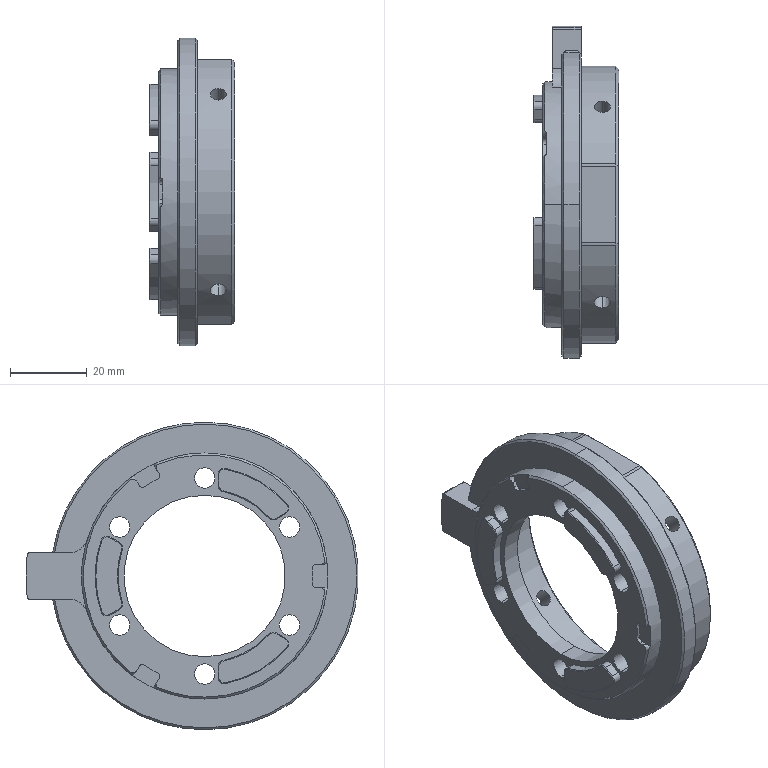NC program | NX | posted with a generic post | part box 22.3 x 86.5 x 80 mm
Lines 2663 to 3025 of 3025:
(PLANAR_MILL_COPY_COPY_COPY_COPY_COPY_COPY_1_COPY_1 , TOOL : D6A45)
N5282 T01 M6
N5284 G54
N5286 G17 G0 G90 X-1.7 Y25.849 S9500 M3
N5288 G43 Z30. H1
N5290 Z0.
N5292 G94 G1 Z-1.5 F1250.
N5294 G3 X-2.2 Y24.983 R1.
N5296 G1 Y23.554
N5298 G2 X-4.486 Y20.72 R2.9
N5300 G3 X-15.701 Y14.245 R21.2
N5302 G2 X-19.299 Y13.682 R2.9
N5304 G1 X-21.774 Y15.111
N5306 G2 X-22.515 Y19.523 R2.9
N5308 X-5.65 Y29.26 R29.8
N5310 X-2.2 Y26.412 R2.9
N5312 G1 Y24.983
N5314 G3 X-1.7 Y24.117 R1.
N5316 G1 Z0.
N5318 G0 Z30.
N5320 X-21.536 Y-14.397
N5322 Z0.
N5324 G1 Z-1.5
N5326 G3 X-20.536 Y-14.397 R1.
N5328 G1 X-19.299 Y-13.682
N5330 G2 X-15.701 Y-14.245 R2.9
N5332 G3 X-4.486 Y-20.72 R21.2
N5334 G2 X-2.2 Y-23.554 R2.9
N5336 G1 Y-26.412
N5338 G2 X-5.65 Y-29.26 R2.9
N5340 X-22.515 Y-19.523 R29.8
N5342 X-21.774 Y-15.111 R2.9
N5344 G1 X-20.536 Y-14.397
N5346 G3 X-20.036 Y-13.531 R1.
N5348 G1 Z0.
N5350 G0 Z30.
N5352 X23.236 Y-11.452
N5354 Z0.
N5356 G1 Z-1.5
N5358 G3 X22.736 Y-10.586 R1.
N5360 G1 X21.499 Y-9.872
N5362 G2 X20.187 Y-6.475 R2.9
N5364 G3 X20.187 Y6.475 R21.2
N5366 G2 X21.499 Y9.872 R2.9
N5368 G1 X23.974 Y11.301
N5370 G2 X28.164 Y9.737 R2.9
N5372 X28.164 Y-9.737 R29.8
N5374 X23.974 Y-11.301 R2.9
N5376 G1 X22.736 Y-10.586
N5378 G3 X21.736 Y-10.586 R1.
N5380 G1 Z0.
N5382 G0 Z30.
(PLANAR_MILL_COPY_COPY_COPY_COPY_COPY_COPY_1_COPY_1_COPY , TOOL : D6A45)
N5384 X13.9 Y25.808
N5386 Z-1.8
N5388 G1 Z-3.3
N5390 G3 X14.4 Y24.942 R1.
N5392 G2 X16.086 Y23.889 R28.8
N5394 G3 X16.371 Y23.955 R0.2
N5396 G1 X16.815 Y24.724
N5398 G2 X17.223 Y25.267 R2.834
N5400 X17.805 Y25.712 R2.371
N5402 X18.641 Y25.948 R1.983
N5404 X19.647 Y25.638 R1.517
N5406 X19.647 Y-25.638 R32.3
N5408 X18.64 Y-25.948 R1.517
N5410 X17.805 Y-25.712 R1.984
N5412 X17.222 Y-25.267 R2.37
N5414 X16.815 Y-24.724 R2.835
N5416 G1 X16.371 Y-23.955
N5418 G3 X16.086 Y-23.889 R0.2
N5420 G2 X12.646 Y-25.875 R28.8
N5422 G3 X12.56 Y-26.155 R0.2
N5424 G1 X13.004 Y-26.924
N5426 G2 X13.271 Y-27.549 R2.834
N5428 X13.365 Y-28.276 R2.371
N5430 X13.152 Y-29.117 R1.983
N5432 X12.38 Y-29.833 R1.517
N5434 X-32.026 Y-4.196 R32.3
N5436 X-31.792 Y-3.169 R1.517
N5438 X-31.17 Y-2.564 R1.984
N5440 X-30.493 Y-2.281 R2.37
N5442 X-29.819 Y-2.2 R2.835
N5444 G1 X-28.931
N5446 G3 X-28.731 Y-1.986 R0.2
N5448 G2 X-28.731 Y1.986 R28.8
N5450 G3 X-28.931 Y2.2 R0.2
N5452 G1 X-29.819
N5454 G2 X-30.494 Y2.282 R2.834
N5456 X-31.17 Y2.564 R2.371
N5458 X-31.792 Y3.169 R1.983
N5460 X-32.026 Y4.196 R1.517
N5462 X12.38 Y29.833 R32.3
N5464 X13.152 Y29.117 R1.517
N5466 X13.365 Y28.275 R1.984
N5468 X13.271 Y27.549 R2.37
N5470 X13.004 Y26.924 R2.835
N5472 G1 X12.56 Y26.155
N5474 G3 X12.646 Y25.875 R0.2
N5476 G2 X14.4 Y24.942 R28.8
N5478 G3 X15.4 Y24.942 R1.
N5480 G1 Z-1.8
N5482 G0 Z30.
(PLANAR_MILL_COPY_COPY_COPY_COPY_COPY_COPY_1_COPY_1_COPY_1 , TOOL : D6A45)
N5484 X1.198 Y25.871
N5486 Z-2.5
N5488 G1 X0.905 Y26.405 Z-2.663
N5490 X0.276 Y26.75 Z-2.855
N5492 X-0.006 Z-2.934
N5494 X0.276 Z-3.009
N5496 X0.905 Y26.405 Z-3.201
N5498 X1.25 Y25.776 Z-3.394
N5500 Y25.225 Z-3.541
N5502 X0.905 Y24.595 Z-3.734
N5504 X0.276 Y24.25 Z-3.926
N5506 X0. Z-4.
N5508 G3 X1.25 Y25.5 R1.25
N5510 X-0.011 Y26.75 R1.25
N5512 X0.545 Y25.919 R1.
N5514 G1 Z-2.5
N5516 G0 Z30.
N5518 X21.151 Y13.604
N5520 Z-2.5
N5522 G1 X20.834 Y13.026 Z-2.677
N5524 X20.863 Y12.364 Z-2.855
N5526 X21.001 Y12.125 Z-2.929
N5528 X20.863 Y12.364 Z-3.003
N5530 X20.834 Y12.475 Z-3.034
N5532 Y12.75 Z-3.107
N5534 Y13.026 Z-3.181
N5536 X21.179 Y13.655 Z-3.374
N5538 X21.808 Y14. Z-3.566
N5540 X22.359 Z-3.714
N5542 X22.729 Y13.856 Z-3.82
N5544 X23.036 Y13.605 Z-3.926
N5546 X23.172 Y13.365 Z-4.
N5548 G3 X21.468 Y13.838 R1.25
N5550 X21.001 Y12.125 R1.25
N5552 X21.501 Y12.991 R1.
N5554 G1 Z-2.5
N5556 G0 Z30.
N5558 X16.662 Y6.951
N5560 Z-2.5
N5562 G1 Z-4.
N5564 X17.284 Y7.212
N5566 G3 X17.89 Y8.007 R1.
N5568 X-2.01 Y19.497 R19.6
N5570 X-2.396 Y18.574 R1.
N5572 G1 X-2.311 Y17.905
N5574 Z-2.5
N5576 G0 Z30.
N5578 X-14.351 Y10.954
N5580 Z-2.5
N5582 G1 Z-4.
N5584 X-14.888 Y11.362
N5586 G3 X-15.879 Y11.489 R1.
N5588 X-15.879 Y-11.489 R19.6
N5590 X-14.888 Y-11.362 R1.
N5592 G1 X-14.351 Y-10.954
N5594 Z-2.5
N5596 G0 Z30.
N5598 X-2.311 Y-17.905
N5600 Z-2.5
N5602 G1 Z-4.
N5604 X-2.396 Y-18.574
N5606 G3 X-2.01 Y-19.497 R1.
N5608 X17.89 Y-8.007 R19.6
N5610 X17.284 Y-7.212 R1.
N5612 G1 X16.662 Y-6.951
N5614 Z-2.5
N5616 G0 Z30.
N5618 X21.827 Y-14.
N5620 Z-2.5
N5622 G1 X22.359 Z-2.643
N5624 X22.729 Y-13.856 Z-2.749
N5626 X23.036 Y-13.605 Z-2.855
N5628 X23.172 Y-13.365 Z-2.929
N5630 X23.036 Y-13.605 Z-3.003
N5632 X22.729 Y-13.856 Z-3.109
N5634 X22.359 Y-14. Z-3.215
N5636 X21.808 Z-3.363
N5638 X21.179 Y-13.655 Z-3.555
N5640 X20.834 Y-13.026 Z-3.748
N5642 X20.863 Y-12.364 Z-3.926
N5644 X21.001 Y-12.125 Z-4.
N5646 G3 X21.459 Y-13.833 R1.25
N5648 X23.172 Y-13.365 R1.25
N5650 X22.174 Y-13.432 R1.
N5652 G1 Z-2.5
N5654 G0 Z30.
N5656 X1.203 Y-25.139
N5658 Z-2.5
N5660 G1 X0.905 Y-24.595 Z-2.666
N5662 X0.276 Y-24.25 Z-2.858
N5664 X0. Z-2.932
N5666 X0.276 Z-3.006
N5668 X0.905 Y-24.595 Z-3.198
N5670 X1.25 Y-25.225 Z-3.391
N5672 Y-25.776 Z-3.538
N5674 X0.905 Y-26.405 Z-3.731
N5676 X0.276 Y-26.75 Z-3.923
N5678 X-0.011 Z-4.
N5680 G3 X1.25 Y-25.511 R1.25
N5682 X0. Y-24.25 R1.25
N5684 X0.5 Y-25.116 R1.
N5686 G1 Z-2.5
N5688 G0 Z30.
N5690 X-23.018 Y-11.898
N5692 Z-2.5
N5694 G1 X-23.334 Y-12.475 Z-2.676
N5696 X-23.3 Y-13.147 Z-2.858
N5698 X-23.161 Y-13.385 Z-2.931
N5700 X-23.3 Y-13.147 Z-3.005
N5702 X-23.334 Y-13.026 Z-3.039
N5704 Y-12.475 Z-3.187
N5706 X-22.989 Y-11.845 Z-3.379
N5708 X-22.359 Y-11.5 Z-3.571
N5710 X-21.808 Z-3.719
N5712 X-21.139 Y-11.886 Z-3.926
N5714 X-21.001 Y-12.125 Z-4.
N5716 G3 X-22.709 Y-11.667 R1.25
N5718 X-23.161 Y-13.385 R1.25
N5720 X-22.719 Y-12.487 R1.
N5722 G1 Z-2.5
N5724 G0 Z30.
N5726 X-22.369 Y11.505
N5728 Z-2.5
N5730 G1 X-21.808 Y11.5 Z-2.651
N5732 X-21.139 Y11.886 Z-2.858
N5734 X-21.001 Y12.125 Z-2.931
N5736 X-21.139 Y11.886 Z-3.005
N5738 X-21.808 Y11.5 Z-3.212
N5740 X-22.359 Z-3.36
N5742 X-22.989 Y11.845 Z-3.552
N5744 X-23.334 Y12.475 Z-3.745
N5746 X-23.3 Y13.147 Z-3.926
N5748 X-23.161 Y13.385 Z-4.
N5750 G3 X-22.718 Y11.673 R1.25
N5752 X-21.001 Y12.125 R1.25
N5754 X-22.001 Y12.125 R1.
N5756 G1 Z-2.5
N5758 G0 Z30.
(DRILLING_COPY_1 , TOOL : D6A45)
N5760 X-22.084 Y12.75 S5000
N5762 G81 G98 Z-5.25 F350. R0.5
N5764 Y-12.75
N5766 X0. Y-25.5
N5768 X22.084 Y-12.75
N5770 Y12.75
N5772 X0. Y25.5
N5774 G80
N5776 G0 X0. Y25.5 Z30.
(PLANAR_MILL_COPY_COPY_COPY_COPY_COPY_COPY_1_COPY_1_COPY_2 , TOOL : D6A45)
N5778 X40.64 Y-10.7 S9500
N5780 Z-7.
N5782 G1 Z-8.5 F1250.
N5784 X40.236 Y-10.
N5786 G3 X39.37 Y-9.5 R1.
N5788 G2 X39.37 Y9.5 R-40.5
N5790 G3 X40.236 Y10. R1.
N5792 G1 X40.64 Y10.7
N5794 Z-7.
N5796 G0 Z30.
(PLANAR_MILL_COPY_COPY_COPY_COPY_COPY_COPY_1_COPY_1_COPY_1_COPY , TOOL : D6A45)
N5798 X35.597 Y8.931
N5800 Z-5.
N5802 G1 Z-6.5
N5804 X35.016 Y8.405
N5806 G3 X34.709 Y7.453 R1.
N5808 X35.327 Y7.4 R3.6
N5810 G1 X45.659
N5812 G2 X47.544 Y5.735 R1.9
N5814 X47.544 Y-5.735 R46.4
N5816 X45.659 Y-7.4 R1.9
N5818 G1 X35.327
N5820 G3 X34.709 Y-7.453 R3.6
N5822 X35.016 Y-8.405 R1.
N5824 G1 X35.597 Y-8.931
N5826 Z-5.
N5828 G0 Z30.
N5830 M5
(TOOLCOMP14_COPY , TOOL : D10JING)
N5832 T14 M6
N5834 G54
N5836 G17 G0 G90 X-7.721 Y33.774 S9500 M3
N5838 G43 Z30. H14
N5840 Z-1.5
N5842 G94 G1 Z-2.5 F1250.
N5844 G41 X-7.67 Y33.688 D14
N5846 X-7.306 Y33.268
N5848 G3 X-6.361 Y32.942 R1.
N5850 G2 X1.55 Y26.412 R6.65
N5852 G1 Y23.554
N5854 G2 X-3.693 Y17.055 R6.65
N5856 G3 X-12.924 Y11.725 R17.45
N5858 G2 X-21.174 Y10.435 R6.65
N5860 G1 X-23.649 Y11.864
N5862 G2 X-25.348 Y21.979 R6.65
N5864 X-6.361 Y32.942 R33.55
N5866 G3 X-5.605 Y33.597 R1.
N5868 G1 X-5.447 Y34.054
N5870 G40
N5872 X-5.431 Y34.153
N5874 Z-1.5
N5876 G0 Z30.
N5878 X19.284 Y14.187
N5880 Z-1.5
N5882 G1 Z-2.5
N5884 G41 X19.361 Y14.123
N5886 X19.861 Y13.834
N5888 G3 X20.861 Y13.834 R1.
N5890 G1 X22.099 Y14.548
N5892 G2 X31.709 Y10.962 R6.65
N5894 X31.709 Y-10.962 R33.55
N5896 X22.099 Y-14.548 R6.65
N5898 G1 X19.624 Y-13.119
N5900 G2 X16.616 Y-5.329 R6.65
N5902 G3 X16.616 Y5.329 R17.45
N5904 G2 X19.624 Y13.119 R6.65
N5906 G1 X20.861 Y13.834
N5908 G3 X21.361 Y14.7 R1.
N5910 G1 Y15.277
N5912 G40
N5914 X21.344 Y15.376
N5916 Z-1.5
N5918 G0 Z30.
N5920 X-4.693 Y-34.149
N5922 Z-1.5
N5924 G1 Z-2.5
N5926 G41 X-4.718 Y-34.053
N5928 X-4.919 Y-33.612
N5930 G3 X-5.733 Y-33.032 R1.
N5932 G2 X-6.361 Y-32.942 R6.65
N5934 X-25.348 Y-21.979 R33.55
N5936 X-23.649 Y-11.864 R6.65
N5938 G1 X-21.174 Y-10.435
N5940 G2 X-12.924 Y-11.725 R6.65
N5942 G3 X-3.693 Y-17.055 R17.45
N5944 G2 X1.55 Y-23.554 R6.65
N5946 G1 Y-26.412
N5948 G2 X-5.733 Y-33.032 R6.65
N5950 G3 X-6.643 Y-33.447 R1.
N5952 G1 X-6.929 Y-33.848
N5954 G40
N5956 X-6.972 Y-33.938
N5958 Z-1.5
N5960 G0 Z30.
N5962 M5
N5964 M2